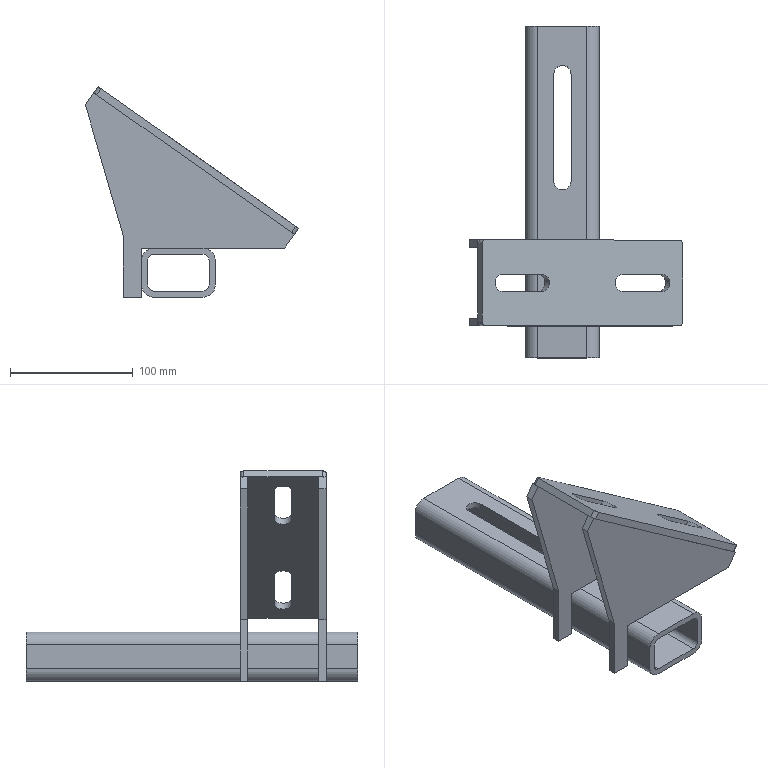Part | STEP file | HL4GZ-1.30.038 (left cane-feed rear mounting seat weldment) | 4 solids | 64 faces | box 173.767 x 270.5 x 171.433 mm | volume 416002 mm3 | plane 44 | cylinder 20 | commonest cylinder face diameters 14 x8 6 x4 10 x4 20 x4